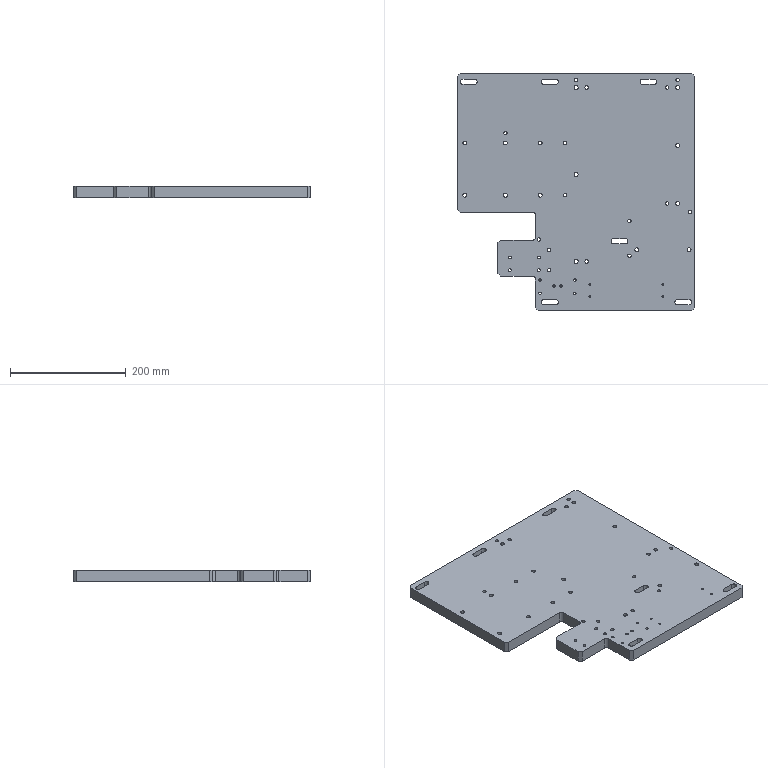CAM job | NX | 3-axis milling, drilling | part box 410 x 410 x 20 mm | stock box 410 x 410 x 20 mm
Tools:
number,name,description,diameter,corner_radius,flute_length,length,flutes
6,D6,平底铣刀-粗,6.0,0.0,25.0,75.0,2
9,D10,平底铣刀-粗,10.0,0.0,35.0,75.0,2
7,D6-J,平底铣刀-精,6.0,0.0,25.0,75.0,2
10,D10-J,平底铣刀-精,10.0,0.0,35.0,75.0,2
2,D6倒角刀,倒角刀,6.0,0.0,3.0,25.0,2
21,M4X0.7,丝锥,3.3,0.0,35.0,50.0,2
22,M5X0.8,丝锥,4.2,0.0,35.0,50.0,2
23,M6X1.0,丝锥,5.0,0.0,35.0,50.0,2
19,M8X1.25,丝锥,6.8,0.0,35.0,50.0,2
18,D6铰刀,Drilling Tool,6.0,0.0,75.0,100.0,6
1,C6定点钻,倒角刀,6.0,0.0,3.0,3.0,2
13,ZT3.4,钻头,3.4,0.0,35.0,50.0,2
15,ZT5.1,钻头,5.1,0.0,35.0,50.0,2
16,ZT6.8,钻头,6.8,0.0,35.0,50.0,2
17,ZT5.9,Drilling Tool,5.9,0.0,35.0,50.0,2
20,ZT4.3,Drilling Tool,4.3,0.0,50.0,75.0,4
Operations:
program,operation,operation_type,tool,method,geometry_group,spindle_rpm,surface_speed,feed_per_tooth,feed_cut,feed_plunge,cut_length_mm,path_length_mm,cut_time_min,machine_time_min
B,DRILL-CHAMFER_2,Operation,D6倒角刀,METHOD,W-B,2000.0,0.0,0.025,100.0,0.0,20.8,319.062,0.208,0.2378
B,DRILL-CHAMFER_3,Operation,D6倒角刀,METHOD,W-B,2000.0,0.0,0.025,100.0,0.0,34.2,294.894,0.342,0.3681
B,MILL-CHAMFER_5,PlanarMilling,D6倒角刀,METHOD,W-B,4000.0,75.398,0.0375,300.0,100.0,72.081,574.901,0.2403,0.2906
B,MILL-CHAMFER_6,PlanarMilling,D6倒角刀,METHOD,W-B,4000.0,75.398,0.075,600.0,100.0,270.305,2794.292,0.4505,0.7029
B,MILL-CHAMFER_7,PlanarMilling,D6倒角刀,METHOD,W-B,4000.0,75.398,0.0375,300.0,100.0,334.815,2933.204,1.116,1.376
B,C0.3-CLOSED-CONTOUR-CHAMFER-6X45L_COPY_2,PlanarMilling,D6倒角刀,WALL-CLIMB_CHAMFER-DEPTH0-STEPG,W-B,4000.0,75.398,0.125,1000.0,100.0,458.625,2024.298,0.4586,0.6152
B,C0.3-CLOSED-CONTOUR-CHAMFER-6X45L_COPY_3,PlanarMilling,D6倒角刀,WALL-CLIMB_CHAMFER-DEPTH0-STEPG,W-B,4000.0,75.398,0.125,1000.0,100.0,1110.091,1575.283,1.11,1.157
A,ZLEVEL-RECIPROCAL-ROUGH-MID_COPY,ZLevelMilling,D10,LAYER-ROUGHING-DEPTHK-STEPG,W-A,3000.0,94.248,0.3833,2300.0,100.0,51618.512,53054.587,22.443,22.586
A,SPOT-DEPTH0.8,Operation,C6定点钻,NONE,W-A,3000.0,56.0,0.01,60.0,90.0,99.0,3731.155,1.65,2.013
A,THROUGH-HOLE-M4-TAP-DRILL,Operation,ZT3.4,NONE,W-A,1500.0,15.551,0.02,60.0,90.0,108.0,487.052,1.8,1.838
A,THROUGH-HOLE-M5-TAP-DRILL,Operation,ZT4.3,NONE,W-A,1200.0,15.834,0.0333,80.0,90.0,162.0,539.516,2.025,2.063
A,THROUGH-HOLE-M6-TAP-DRILL,Operation,ZT5.1,NONE,W-A,800.0,12.566,0.0625,100.0,90.0,112.0,421.055,1.12,1.151
A,THROUGH-HOLE-6.0-FINISH-PRE-DRILL,Operation,ZT5.9,NONE,W-A,1000.0,18.535,0.04,80.0,90.0,385.548,1880.092,4.819,4.969
A,THROUGH-HOLE-M8-TAP-DRILL,Operation,ZT6.8,NONE,W-A,600.0,12.818,0.1,120.0,90.0,742.116,4272.21,6.184,6.537
A,THROUGH-SLOT-ROUGH_1,VolumeBased25DMillingOperation,D6,METHOD,W-A,3000.0,188.0,0.2,1200.0,100.0,24309.952,25996.335,20.258,20.427
A,SLOT-FINISH_1,VolumeBased25DMillingOperation,D6-J,METHOD,W-A,3200.0,32.0,0.1143,600.0,100.0,1239.674,3263.874,2.066,2.268
A,DRILL-CHAMFER_1,Operation,D6倒角刀,METHOD,W-A,4000.0,75.398,0.01,80.0,0.0,20.8,319.062,0.26,0.2898
A,MILL-CHAMFER_1,PlanarMilling,D6倒角刀,METHOD,W-A,4000.0,75.398,0.025,200.0,100.0,108.122,824.658,0.5406,0.6123
A,MILL-CHAMFER_2,PlanarMilling,D6倒角刀,METHOD,W-A,4000.0,75.398,0.0375,300.0,100.0,79.753,578.594,0.2658,0.3157
A,MILL-CHAMFER_3,PlanarMilling,D6倒角刀,METHOD,W-A,4000.0,75.398,0.05,400.0,100.0,314.456,2818.088,0.7861,1.036
A,MILL-CHAMFER_4,PlanarMilling,D6倒角刀,METHOD,W-A,4000.0,75.398,0.0625,500.0,100.0,328.678,2919.36,0.6574,0.9164
A,C0.3-CLOSED-CONTOUR-CHAMFER-6X45L_COPY,PlanarMilling,D6倒角刀,WALL-CLIMB_CHAMFER-DEPTH0-STEPG,W-A,4000.0,75.398,0.125,1000.0,100.0,462.656,1995.005,0.4627,0.6159
A,C0.3-CLOSED-CONTOUR-CHAMFER-6X45L_COPY_1,PlanarMilling,D6倒角刀,WALL-CLIMB_CHAMFER-DEPTH0-STEPG,W-A,4000.0,75.398,0.125,1000.0,100.0,1110.091,1575.283,1.11,1.157
A,REAM-HOLE,Operation,D6铰刀,METHOD,W-A,500.0,9.425,0.0167,50.0,0.0,330.0,1768.996,6.6,6.744
A,THROUGH-HOLE-TAP-M4,Operation,M4X0.7,METHOD,W-A,500.0,5.184,0.0007,0.7,90.0,98.0,467.052,140.0,140.037
A,THROUGH-HOLE-TAP-M6,Operation,M6X1.0,METHOD,W-A,400.0,6.283,0.0013,1.0,90.0,98.0,393.055,98.0,98.029
A,THROUGH-HOLE-TAP-M5,Operation,M5X0.8,METHOD,W-A,500.0,6.597,0.0008,0.8,90.0,147.0,509.516,183.75,183.786
A,THROUGH-HOLE-TAP-M8,Operation,M8X1.25,METHOD,W-A,300.0,6.409,0.0021,1.25,90.0,357.0,1991.782,285.6,285.764
A,FLOOR-WALL-FINISH-SIDE-MID_COPY,VolumeBased25DMillingOperation,D6-J,SIDE-FINISHING-DEPTHK-STEPG,W-A,3500.0,65.972,0.1143,800.0,100.0,879.702,1365.119,1.1,1.148
A,FLOOR-WALL-FINISH-SIDE-MID_COPY_1,VolumeBased25DMillingOperation,D10-J,SIDE-FINISHING-DEPTHK-STEPG,W-A,3000.0,94.245,0.1333,800.0,100.0,151.119,1456.222,0.1889,0.3194